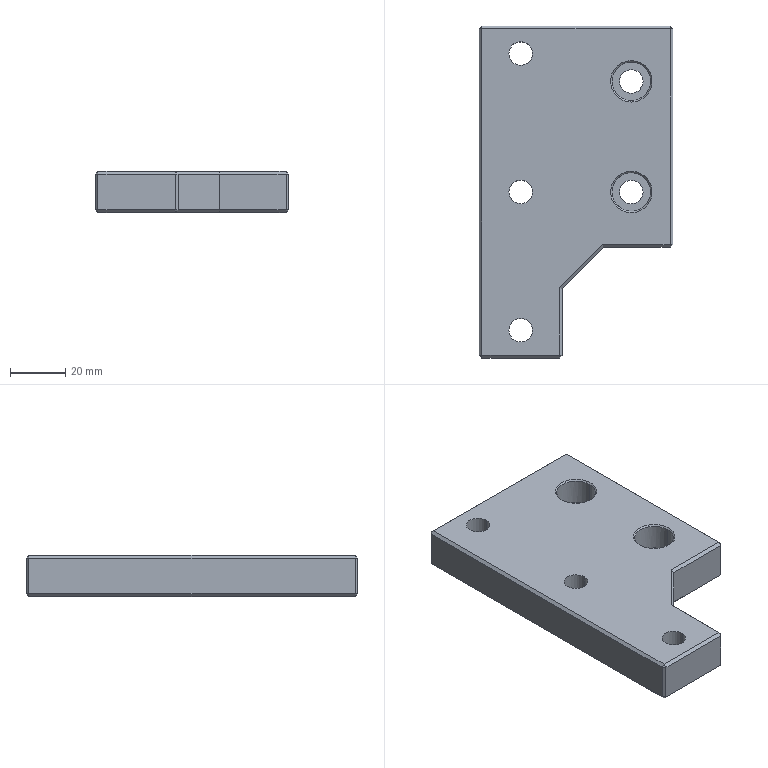Part | STEP file | Roller base fixing plate | 1 solid | 83 faces | box 70 x 120 x 15 mm | volume 94561 mm3 | plane 43 | cone 20 | cylinder 20 | commonest cylinder face diameters 8.5 x10 14 x10